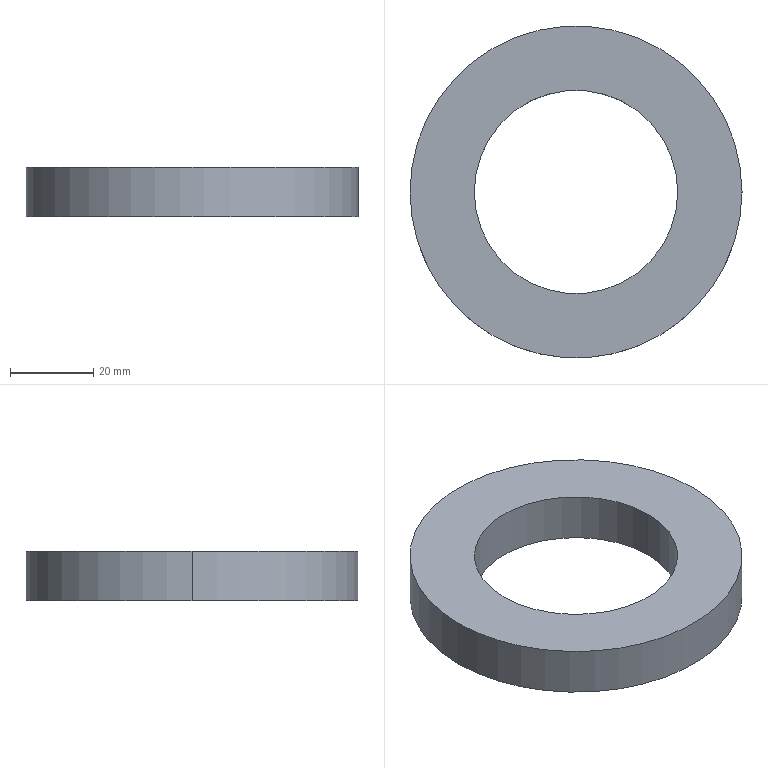Part | STEP file | BB013A02M-04-37A | 1 solid | 6 faces | box 80 x 80 x 12 mm | volume 37690 mm3 | cylinder 4 | plane 2 | commonest cylinder face diameters 49 x2 80 x2
STEP:
#1=CARTESIAN_POINT('',(0.,0.,0.));
#2=DIRECTION('',(0.,0.,1.));
#3=DIRECTION('',(1.,0.,0.));
#4=AXIS2_PLACEMENT_3D('',#1,#2,#3);
#5=CARTESIAN_POINT('',(-24.5,0.,12.));
#6=VERTEX_POINT('',#5);
#7=CARTESIAN_POINT('',(-24.5,0.,0.));
#8=VERTEX_POINT('',#7);
#9=CARTESIAN_POINT('',(-24.5,0.,12.));
#10=DIRECTION('',(0.,0.,-1.));
#11=VECTOR('',#10,1.);
#12=LINE('',#9,#11);
#13=CARTESIAN_POINT('',(0.,0.,12.));
#14=DIRECTION('',(0.,0.,-1.));
#15=DIRECTION('',(-1.,0.,0.));
#16=AXIS2_PLACEMENT_3D('',#13,#14,#15);
#17=CYLINDRICAL_SURFACE('',#16,24.5);
#18=CARTESIAN_POINT('',(6.283,0.));
#19=DIRECTION('',(0.,1.));
#20=VECTOR('',#19,1.);
#21=LINE('',#18,#20);
#22=(GEOMETRIC_REPRESENTATION_CONTEXT(2)PARAMETRIC_REPRESENTATION_CONTEXT()REPRESENTATION_CONTEXT('',''));
#23=DEFINITIONAL_REPRESENTATION('',(#21),#22);
#24=PCURVE('',#17,#23);
#25=CARTESIAN_POINT('',(0.,0.,12.));
#26=DIRECTION('',(0.,0.,-1.));
#27=DIRECTION('',(-1.,0.,0.));
#28=AXIS2_PLACEMENT_3D('',#25,#26,#27);
#29=CYLINDRICAL_SURFACE('',#28,24.5);
#30=CARTESIAN_POINT('',(0.,0.));
#31=DIRECTION('',(0.,1.));
#32=VECTOR('',#31,1.);
#33=LINE('',#30,#32);
#34=(GEOMETRIC_REPRESENTATION_CONTEXT(2)PARAMETRIC_REPRESENTATION_CONTEXT()REPRESENTATION_CONTEXT('',''));
#35=DEFINITIONAL_REPRESENTATION('',(#33),#34);
#36=PCURVE('',#29,#35);
#37=SURFACE_CURVE('',#12,(#24,#36),.PCURVE_S1.);
#38=EDGE_CURVE('',#6,#8,#37,.T.);
#39=ORIENTED_EDGE('',*,*,#38,.T.);
#40=CARTESIAN_POINT('',(24.5,0.,0.));
#41=VERTEX_POINT('',#40);
#42=CARTESIAN_POINT('',(0.,0.,0.));
#43=DIRECTION('',(0.,0.,1.));
#44=DIRECTION('',(-1.,0.,0.));
#45=AXIS2_PLACEMENT_3D('',#42,#43,#44);
#46=CIRCLE('',#45,24.5);
#47=CARTESIAN_POINT('',(6.283,12.));
#48=DIRECTION('',(-1.,0.));
#49=VECTOR('',#48,1.);
#50=LINE('',#47,#49);
#51=(GEOMETRIC_REPRESENTATION_CONTEXT(2)PARAMETRIC_REPRESENTATION_CONTEXT()REPRESENTATION_CONTEXT('',''));
#52=DEFINITIONAL_REPRESENTATION('',(#50),#51);
#53=PCURVE('',#17,#52);
#54=CARTESIAN_POINT('',(0.,0.,0.));
#55=DIRECTION('',(0.,0.,1.));
#56=DIRECTION('',(1.,0.,0.));
#57=AXIS2_PLACEMENT_3D('',#54,#55,#56);
#58=PLANE('',#57);
#59=CARTESIAN_POINT('',(0.,0.));
#60=DIRECTION('',(-1.,0.));
#61=AXIS2_PLACEMENT_2D('',#59,#60);
#62=CIRCLE('',#61,24.5);
#63=(GEOMETRIC_REPRESENTATION_CONTEXT(2)PARAMETRIC_REPRESENTATION_CONTEXT()REPRESENTATION_CONTEXT('',''));
#64=DEFINITIONAL_REPRESENTATION('',(#62),#63);
#65=PCURVE('',#58,#64);
#66=SURFACE_CURVE('',#46,(#53,#65),.PCURVE_S1.);
#67=EDGE_CURVE('',#8,#41,#66,.T.);
#68=ORIENTED_EDGE('',*,*,#67,.T.);
#69=CARTESIAN_POINT('',(24.5,0.,12.));
#70=VERTEX_POINT('',#69);
#71=CARTESIAN_POINT('',(24.5,0.,12.));
#72=DIRECTION('',(0.,0.,-1.));
#73=VECTOR('',#72,1.);
#74=LINE('',#71,#73);
#75=CARTESIAN_POINT('',(3.142,0.));
#76=DIRECTION('',(0.,1.));
#77=VECTOR('',#76,1.);
#78=LINE('',#75,#77);
#79=(GEOMETRIC_REPRESENTATION_CONTEXT(2)PARAMETRIC_REPRESENTATION_CONTEXT()REPRESENTATION_CONTEXT('',''));
#80=DEFINITIONAL_REPRESENTATION('',(#78),#79);
#81=PCURVE('',#17,#80);
#82=CARTESIAN_POINT('',(3.142,0.));
#83=DIRECTION('',(0.,1.));
#84=VECTOR('',#83,1.);
#85=LINE('',#82,#84);
#86=(GEOMETRIC_REPRESENTATION_CONTEXT(2)PARAMETRIC_REPRESENTATION_CONTEXT()REPRESENTATION_CONTEXT('',''));
#87=DEFINITIONAL_REPRESENTATION('',(#85),#86);
#88=PCURVE('',#29,#87);
#89=SURFACE_CURVE('',#74,(#81,#88),.PCURVE_S1.);
#90=EDGE_CURVE('',#70,#41,#89,.T.);
#91=ORIENTED_EDGE('',*,*,#90,.F.);
#92=CARTESIAN_POINT('',(0.,0.,12.));
#93=DIRECTION('',(0.,0.,-1.));
#94=DIRECTION('',(-1.,0.,0.));
#95=AXIS2_PLACEMENT_3D('',#92,#93,#94);
#96=CIRCLE('',#95,24.5);
#97=CARTESIAN_POINT('',(0.,0.));
#98=DIRECTION('',(1.,0.));
#99=VECTOR('',#98,1.);
#100=LINE('',#97,#99);
#101=(GEOMETRIC_REPRESENTATION_CONTEXT(2)PARAMETRIC_REPRESENTATION_CONTEXT()REPRESENTATION_CONTEXT('',''));
#102=DEFINITIONAL_REPRESENTATION('',(#100),#101);
#103=PCURVE('',#17,#102);
#104=CARTESIAN_POINT('',(0.,0.,12.));
#105=DIRECTION('',(0.,0.,1.));
#106=DIRECTION('',(1.,0.,0.));
#107=AXIS2_PLACEMENT_3D('',#104,#105,#106);
#108=PLANE('',#107);
#109=CARTESIAN_POINT('',(-24.5,0.));
#110=CARTESIAN_POINT('',(-24.5,42.435));
#111=CARTESIAN_POINT('',(12.25,21.218));
#112=CARTESIAN_POINT('',(49.,0.));
#113=CARTESIAN_POINT('',(12.25,-21.218));
#114=CARTESIAN_POINT('',(-24.5,-42.435));
#115=CARTESIAN_POINT('',(-24.5,0.));
#116=(BOUNDED_CURVE()B_SPLINE_CURVE(2,(#109,#110,#111,#112,#113,#114,#115),.UNSPECIFIED.,.T.,.F.)B_SPLINE_CURVE_WITH_KNOTS((1,2,2,2,2,1),(-2.094,0.,2.094,4.189,6.283,8.378),.UNSPECIFIED.)CURVE()GEOMETRIC_REPRESENTATION_ITEM()RATIONAL_B_SPLINE_CURVE((1.,0.5,1.,0.5,1.,0.5,1.))REPRESENTATION_ITEM(''));
#117=(GEOMETRIC_REPRESENTATION_CONTEXT(2)PARAMETRIC_REPRESENTATION_CONTEXT()REPRESENTATION_CONTEXT('',''));
#118=DEFINITIONAL_REPRESENTATION('',(#116),#117);
#119=PCURVE('',#108,#118);
#120=SURFACE_CURVE('',#96,(#103,#119),.PCURVE_S1.);
#121=EDGE_CURVE('',#70,#6,#120,.T.);
#122=ORIENTED_EDGE('',*,*,#121,.T.);
#123=EDGE_LOOP('',(#39,#68,#91,#122));
#124=FACE_BOUND('',#123,.F.);
#125=ADVANCED_FACE('',(#124),#17,.F.);
#126=CARTESIAN_POINT('',(40.,0.,12.));
#127=VERTEX_POINT('',#126);
#128=CARTESIAN_POINT('',(-40.,0.,12.));
#129=VERTEX_POINT('',#128);
#130=CARTESIAN_POINT('',(0.,0.,12.));
#131=DIRECTION('',(0.,0.,1.));
#132=DIRECTION('',(-1.,0.,0.));
#133=AXIS2_PLACEMENT_3D('',#130,#131,#132);
#134=CIRCLE('',#133,40.);
#135=CARTESIAN_POINT('',(0.,0.,12.));
#136=DIRECTION('',(0.,0.,-1.));
#137=DIRECTION('',(-1.,0.,0.));
#138=AXIS2_PLACEMENT_3D('',#135,#136,#137);
#139=CYLINDRICAL_SURFACE('',#138,40.);
#140=CARTESIAN_POINT('',(6.283,0.));
#141=DIRECTION('',(-1.,0.));
#142=VECTOR('',#141,1.);
#143=LINE('',#140,#142);
#144=(GEOMETRIC_REPRESENTATION_CONTEXT(2)PARAMETRIC_REPRESENTATION_CONTEXT()REPRESENTATION_CONTEXT('',''));
#145=DEFINITIONAL_REPRESENTATION('',(#143),#144);
#146=PCURVE('',#139,#145);
#147=CARTESIAN_POINT('',(0.,0.));
#148=DIRECTION('',(-1.,0.));
#149=AXIS2_PLACEMENT_2D('',#147,#148);
#150=CIRCLE('',#149,40.);
#151=(GEOMETRIC_REPRESENTATION_CONTEXT(2)PARAMETRIC_REPRESENTATION_CONTEXT()REPRESENTATION_CONTEXT('',''));
#152=DEFINITIONAL_REPRESENTATION('',(#150),#151);
#153=PCURVE('',#108,#152);
#154=SURFACE_CURVE('',#134,(#146,#153),.PCURVE_S1.);
#155=EDGE_CURVE('',#127,#129,#154,.T.);
#156=ORIENTED_EDGE('',*,*,#155,.F.);
#157=CARTESIAN_POINT('',(40.,0.,0.));
#158=VERTEX_POINT('',#157);
#159=CARTESIAN_POINT('',(40.,0.,12.));
#160=DIRECTION('',(0.,0.,-1.));
#161=VECTOR('',#160,1.);
#162=LINE('',#159,#161);
#163=CARTESIAN_POINT('',(3.142,0.));
#164=DIRECTION('',(0.,1.));
#165=VECTOR('',#164,1.);
#166=LINE('',#163,#165);
#167=(GEOMETRIC_REPRESENTATION_CONTEXT(2)PARAMETRIC_REPRESENTATION_CONTEXT()REPRESENTATION_CONTEXT('',''));
#168=DEFINITIONAL_REPRESENTATION('',(#166),#167);
#169=PCURVE('',#139,#168);
#170=CARTESIAN_POINT('',(0.,0.,12.));
#171=DIRECTION('',(0.,0.,-1.));
#172=DIRECTION('',(-1.,0.,0.));
#173=AXIS2_PLACEMENT_3D('',#170,#171,#172);
#174=CYLINDRICAL_SURFACE('',#173,40.);
#175=CARTESIAN_POINT('',(3.142,0.));
#176=DIRECTION('',(0.,1.));
#177=VECTOR('',#176,1.);
#178=LINE('',#175,#177);
#179=(GEOMETRIC_REPRESENTATION_CONTEXT(2)PARAMETRIC_REPRESENTATION_CONTEXT()REPRESENTATION_CONTEXT('',''));
#180=DEFINITIONAL_REPRESENTATION('',(#178),#179);
#181=PCURVE('',#174,#180);
#182=SURFACE_CURVE('',#162,(#169,#181),.PCURVE_S1.);
#183=EDGE_CURVE('',#127,#158,#182,.T.);
#184=ORIENTED_EDGE('',*,*,#183,.T.);
#185=CARTESIAN_POINT('',(-40.,0.,0.));
#186=VERTEX_POINT('',#185);
#187=CARTESIAN_POINT('',(0.,0.,0.));
#188=DIRECTION('',(0.,0.,1.));
#189=DIRECTION('',(-1.,0.,0.));
#190=AXIS2_PLACEMENT_3D('',#187,#188,#189);
#191=CIRCLE('',#190,40.);
#192=CARTESIAN_POINT('',(6.283,12.));
#193=DIRECTION('',(-1.,0.));
#194=VECTOR('',#193,1.);
#195=LINE('',#192,#194);
#196=(GEOMETRIC_REPRESENTATION_CONTEXT(2)PARAMETRIC_REPRESENTATION_CONTEXT()REPRESENTATION_CONTEXT('',''));
#197=DEFINITIONAL_REPRESENTATION('',(#195),#196);
#198=PCURVE('',#139,#197);
#199=CARTESIAN_POINT('',(0.,0.));
#200=DIRECTION('',(-1.,0.));
#201=AXIS2_PLACEMENT_2D('',#199,#200);
#202=CIRCLE('',#201,40.);
#203=(GEOMETRIC_REPRESENTATION_CONTEXT(2)PARAMETRIC_REPRESENTATION_CONTEXT()REPRESENTATION_CONTEXT('',''));
#204=DEFINITIONAL_REPRESENTATION('',(#202),#203);
#205=PCURVE('',#58,#204);
#206=SURFACE_CURVE('',#191,(#198,#205),.PCURVE_S1.);
#207=EDGE_CURVE('',#158,#186,#206,.T.);
#208=ORIENTED_EDGE('',*,*,#207,.T.);
#209=CARTESIAN_POINT('',(-40.,0.,12.));
#210=DIRECTION('',(0.,0.,-1.));
#211=VECTOR('',#210,1.);
#212=LINE('',#209,#211);
#213=CARTESIAN_POINT('',(0.,0.));
#214=DIRECTION('',(0.,1.));
#215=VECTOR('',#214,1.);
#216=LINE('',#213,#215);
#217=(GEOMETRIC_REPRESENTATION_CONTEXT(2)PARAMETRIC_REPRESENTATION_CONTEXT()REPRESENTATION_CONTEXT('',''));
#218=DEFINITIONAL_REPRESENTATION('',(#216),#217);
#219=PCURVE('',#139,#218);
#220=CARTESIAN_POINT('',(6.283,0.));
#221=DIRECTION('',(0.,1.));
#222=VECTOR('',#221,1.);
#223=LINE('',#220,#222);
#224=(GEOMETRIC_REPRESENTATION_CONTEXT(2)PARAMETRIC_REPRESENTATION_CONTEXT()REPRESENTATION_CONTEXT('',''));
#225=DEFINITIONAL_REPRESENTATION('',(#223),#224);
#226=PCURVE('',#174,#225);
#227=SURFACE_CURVE('',#212,(#219,#226),.PCURVE_S1.);
#228=EDGE_CURVE('',#129,#186,#227,.T.);
#229=ORIENTED_EDGE('',*,*,#228,.F.);
#230=EDGE_LOOP('',(#156,#184,#208,#229));
#231=FACE_BOUND('',#230,.T.);
#232=ADVANCED_FACE('',(#231),#139,.T.);
#233=CARTESIAN_POINT('',(0.,0.,12.));
#234=DIRECTION('',(0.,0.,-1.));
#235=DIRECTION('',(-1.,0.,0.));
#236=AXIS2_PLACEMENT_3D('',#233,#234,#235);
#237=CIRCLE('',#236,24.5);
#238=CARTESIAN_POINT('',(-24.5,0.));
#239=CARTESIAN_POINT('',(-24.5,42.435));
#240=CARTESIAN_POINT('',(12.25,21.218));
#241=CARTESIAN_POINT('',(49.,0.));
#242=CARTESIAN_POINT('',(12.25,-21.218));
#243=CARTESIAN_POINT('',(-24.5,-42.435));
#244=CARTESIAN_POINT('',(-24.5,0.));
#245=(BOUNDED_CURVE()B_SPLINE_CURVE(2,(#238,#239,#240,#241,#242,#243,#244),.UNSPECIFIED.,.T.,.F.)B_SPLINE_CURVE_WITH_KNOTS((1,2,2,2,2,1),(-2.094,0.,2.094,4.189,6.283,8.378),.UNSPECIFIED.)CURVE()GEOMETRIC_REPRESENTATION_ITEM()RATIONAL_B_SPLINE_CURVE((1.,0.5,1.,0.5,1.,0.5,1.))REPRESENTATION_ITEM(''));
#246=(GEOMETRIC_REPRESENTATION_CONTEXT(2)PARAMETRIC_REPRESENTATION_CONTEXT()REPRESENTATION_CONTEXT('',''));
#247=DEFINITIONAL_REPRESENTATION('',(#245),#246);
#248=PCURVE('',#108,#247);
#249=CARTESIAN_POINT('',(0.,0.));
#250=DIRECTION('',(1.,0.));
#251=VECTOR('',#250,1.);
#252=LINE('',#249,#251);
#253=(GEOMETRIC_REPRESENTATION_CONTEXT(2)PARAMETRIC_REPRESENTATION_CONTEXT()REPRESENTATION_CONTEXT('',''));
#254=DEFINITIONAL_REPRESENTATION('',(#252),#253);
#255=PCURVE('',#29,#254);
#256=SURFACE_CURVE('',#237,(#248,#255),.PCURVE_S1.);
#257=EDGE_CURVE('',#6,#70,#256,.T.);
#258=ORIENTED_EDGE('',*,*,#257,.T.);
#259=ORIENTED_EDGE('',*,*,#121,.T.);
#260=EDGE_LOOP('',(#258,#259));
#261=FACE_BOUND('',#260,.T.);
#262=CARTESIAN_POINT('',(0.,0.,12.));
#263=DIRECTION('',(0.,0.,1.));
#264=DIRECTION('',(-1.,0.,0.));
#265=AXIS2_PLACEMENT_3D('',#262,#263,#264);
#266=CIRCLE('',#265,40.);
#267=CARTESIAN_POINT('',(0.,0.));
#268=DIRECTION('',(-1.,0.));
#269=AXIS2_PLACEMENT_2D('',#267,#268);
#270=CIRCLE('',#269,40.);
#271=(GEOMETRIC_REPRESENTATION_CONTEXT(2)PARAMETRIC_REPRESENTATION_CONTEXT()REPRESENTATION_CONTEXT('',''));
#272=DEFINITIONAL_REPRESENTATION('',(#270),#271);
#273=PCURVE('',#108,#272);
#274=CARTESIAN_POINT('',(6.283,0.));
#275=DIRECTION('',(-1.,0.));
#276=VECTOR('',#275,1.);
#277=LINE('',#274,#276);
#278=(GEOMETRIC_REPRESENTATION_CONTEXT(2)PARAMETRIC_REPRESENTATION_CONTEXT()REPRESENTATION_CONTEXT('',''));
#279=DEFINITIONAL_REPRESENTATION('',(#277),#278);
#280=PCURVE('',#174,#279);
#281=SURFACE_CURVE('',#266,(#273,#280),.PCURVE_S1.);
#282=EDGE_CURVE('',#129,#127,#281,.T.);
#283=ORIENTED_EDGE('',*,*,#282,.T.);
#284=ORIENTED_EDGE('',*,*,#155,.T.);
#285=EDGE_LOOP('',(#283,#284));
#286=FACE_BOUND('',#285,.T.);
#287=ADVANCED_FACE('',(#261,#286),#108,.T.);
#288=CARTESIAN_POINT('',(0.,0.,0.));
#289=DIRECTION('',(0.,0.,1.));
#290=DIRECTION('',(-1.,0.,0.));
#291=AXIS2_PLACEMENT_3D('',#288,#289,#290);
#292=CIRCLE('',#291,24.5);
#293=CARTESIAN_POINT('',(6.283,12.));
#294=DIRECTION('',(-1.,0.));
#295=VECTOR('',#294,1.);
#296=LINE('',#293,#295);
#297=(GEOMETRIC_REPRESENTATION_CONTEXT(2)PARAMETRIC_REPRESENTATION_CONTEXT()REPRESENTATION_CONTEXT('',''));
#298=DEFINITIONAL_REPRESENTATION('',(#296),#297);
#299=PCURVE('',#29,#298);
#300=CARTESIAN_POINT('',(0.,0.));
#301=DIRECTION('',(-1.,0.));
#302=AXIS2_PLACEMENT_2D('',#300,#301);
#303=CIRCLE('',#302,24.5);
#304=(GEOMETRIC_REPRESENTATION_CONTEXT(2)PARAMETRIC_REPRESENTATION_CONTEXT()REPRESENTATION_CONTEXT('',''));
#305=DEFINITIONAL_REPRESENTATION('',(#303),#304);
#306=PCURVE('',#58,#305);
#307=SURFACE_CURVE('',#292,(#299,#306),.PCURVE_S1.);
#308=EDGE_CURVE('',#41,#8,#307,.T.);
#309=ORIENTED_EDGE('',*,*,#308,.T.);
#310=ORIENTED_EDGE('',*,*,#38,.F.);
#311=ORIENTED_EDGE('',*,*,#257,.T.);
#312=ORIENTED_EDGE('',*,*,#90,.T.);
#313=EDGE_LOOP('',(#309,#310,#311,#312));
#314=FACE_BOUND('',#313,.F.);
#315=ADVANCED_FACE('',(#314),#29,.F.);
#316=ORIENTED_EDGE('',*,*,#183,.F.);
#317=ORIENTED_EDGE('',*,*,#282,.F.);
#318=ORIENTED_EDGE('',*,*,#228,.T.);
#319=CARTESIAN_POINT('',(0.,0.,0.));
#320=DIRECTION('',(0.,0.,1.));
#321=DIRECTION('',(-1.,0.,0.));
#322=AXIS2_PLACEMENT_3D('',#319,#320,#321);
#323=CIRCLE('',#322,40.);
#324=CARTESIAN_POINT('',(6.283,12.));
#325=DIRECTION('',(-1.,0.));
#326=VECTOR('',#325,1.);
#327=LINE('',#324,#326);
#328=(GEOMETRIC_REPRESENTATION_CONTEXT(2)PARAMETRIC_REPRESENTATION_CONTEXT()REPRESENTATION_CONTEXT('',''));
#329=DEFINITIONAL_REPRESENTATION('',(#327),#328);
#330=PCURVE('',#174,#329);
#331=CARTESIAN_POINT('',(0.,0.));
#332=DIRECTION('',(-1.,0.));
#333=AXIS2_PLACEMENT_2D('',#331,#332);
#334=CIRCLE('',#333,40.);
#335=(GEOMETRIC_REPRESENTATION_CONTEXT(2)PARAMETRIC_REPRESENTATION_CONTEXT()REPRESENTATION_CONTEXT('',''));
#336=DEFINITIONAL_REPRESENTATION('',(#334),#335);
#337=PCURVE('',#58,#336);
#338=SURFACE_CURVE('',#323,(#330,#337),.PCURVE_S1.);
#339=EDGE_CURVE('',#186,#158,#338,.T.);
#340=ORIENTED_EDGE('',*,*,#339,.T.);
#341=EDGE_LOOP('',(#316,#317,#318,#340));
#342=FACE_BOUND('',#341,.T.);
#343=ADVANCED_FACE('',(#342),#174,.T.);
#344=ORIENTED_EDGE('',*,*,#67,.T.);
#345=ORIENTED_EDGE('',*,*,#308,.T.);
#346=EDGE_LOOP('',(#344,#345));
#347=FACE_BOUND('',#346,.T.);
#348=ORIENTED_EDGE('',*,*,#339,.F.);
#349=ORIENTED_EDGE('',*,*,#207,.F.);
#350=EDGE_LOOP('',(#348,#349));
#351=FACE_BOUND('',#350,.T.);
#352=ADVANCED_FACE('',(#347,#351),#58,.F.);
#353=CLOSED_SHELL('',(#125,#232,#287,#315,#343,#352));
#354=MANIFOLD_SOLID_BREP('',#353);
#355=(LENGTH_UNIT()NAMED_UNIT(*)SI_UNIT(.MILLI.,.METRE.));
#356=UNCERTAINTY_MEASURE_WITH_UNIT(LENGTH_MEASURE(0.0000001),#355,'','');
#357=(NAMED_UNIT(*)PLANE_ANGLE_UNIT()SI_UNIT($,.RADIAN.));
#358=(NAMED_UNIT(*)SI_UNIT($,.STERADIAN.)SOLID_ANGLE_UNIT());
#359=(GEOMETRIC_REPRESENTATION_CONTEXT(3)GLOBAL_UNCERTAINTY_ASSIGNED_CONTEXT((#356))GLOBAL_UNIT_ASSIGNED_CONTEXT((#355,#357,#358))REPRESENTATION_CONTEXT('',''));
#360=ADVANCED_BREP_SHAPE_REPRESENTATION('',(#4,#354),#359);